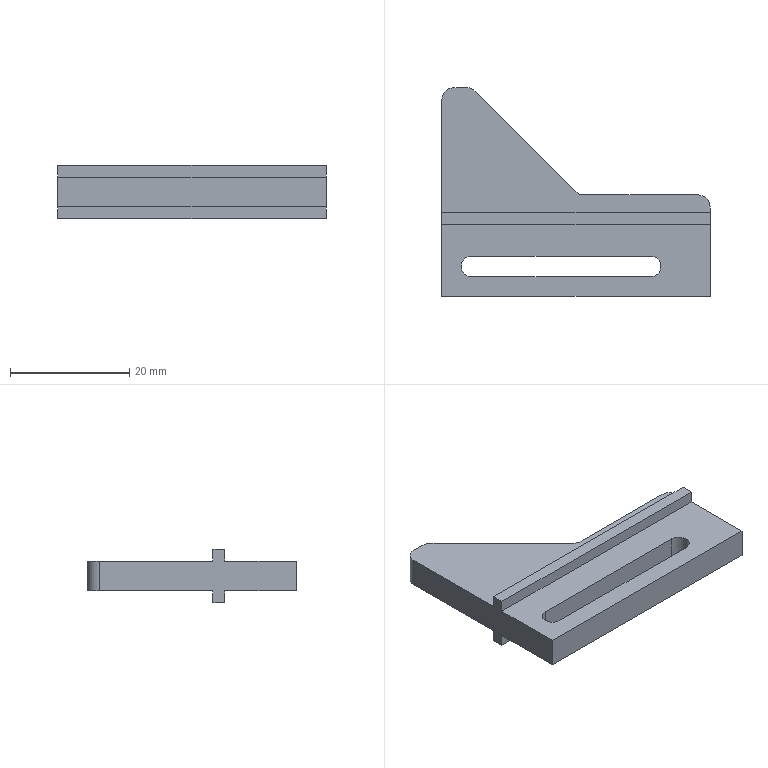Part | NX | 1 solid | 24 faces | box 45 x 35 x 9 mm | volume 4863 mm3 | plane 18 | cylinder 6 | commonest cylinder face diameters 4 x4 3.5 x2
STEP:
#1=CARTESIAN_POINT('',(-10.,-10.25,2.5));
#2=VERTEX_POINT('',#1);
#3=CARTESIAN_POINT('',(-10.,-13.75,2.5));
#4=VERTEX_POINT('',#3);
#5=CARTESIAN_POINT('',(-10.,-12.,2.5));
#6=DIRECTION('',(0.,0.,-1.));
#7=DIRECTION('',(-1.,0.,0.));
#8=AXIS2_PLACEMENT_3D('',#5,#6,#7);
#9=CIRCLE('',#8,1.75);
#10=EDGE_CURVE('',#2,#4,#9,.T.);
#11=ORIENTED_EDGE('',*,*,#10,.T.);
#12=CARTESIAN_POINT('',(-40.,-13.75,2.5));
#13=VERTEX_POINT('',#12);
#14=CARTESIAN_POINT('',(-10.,-13.75,2.5));
#15=DIRECTION('',(-1.,0.,0.));
#16=VECTOR('',#15,1000.);
#17=LINE('',#14,#16);
#18=EDGE_CURVE('',#4,#13,#17,.T.);
#19=ORIENTED_EDGE('',*,*,#18,.T.);
#20=CARTESIAN_POINT('',(-40.,-10.25,2.5));
#21=VERTEX_POINT('',#20);
#22=CARTESIAN_POINT('',(-40.,-12.,2.5));
#23=DIRECTION('',(0.,0.,-1.));
#24=DIRECTION('',(-1.,0.,0.));
#25=AXIS2_PLACEMENT_3D('',#22,#23,#24);
#26=CIRCLE('',#25,1.75);
#27=EDGE_CURVE('',#13,#21,#26,.T.);
#28=ORIENTED_EDGE('',*,*,#27,.T.);
#29=CARTESIAN_POINT('',(-10.,-10.25,2.5));
#30=DIRECTION('',(1.,0.,0.));
#31=VECTOR('',#30,1000.);
#32=LINE('',#29,#31);
#33=EDGE_CURVE('',#21,#2,#32,.T.);
#34=ORIENTED_EDGE('',*,*,#33,.T.);
#35=EDGE_LOOP('',(#11,#19,#28,#34));
#36=FACE_BOUND('',#35,.T.);
#37=CARTESIAN_POINT('',(0.,-17.,2.5));
#38=VERTEX_POINT('',#37);
#39=CARTESIAN_POINT('',(0.,-5.,2.5));
#40=VERTEX_POINT('',#39);
#41=CARTESIAN_POINT('',(0.,-17.,2.5));
#42=DIRECTION('',(0.,1.,0.));
#43=VECTOR('',#42,1000.);
#44=LINE('',#41,#43);
#45=EDGE_CURVE('',#38,#40,#44,.T.);
#46=ORIENTED_EDGE('',*,*,#45,.T.);
#47=CARTESIAN_POINT('',(-45.,-5.,2.5));
#48=VERTEX_POINT('',#47);
#49=CARTESIAN_POINT('',(0.,-5.,2.5));
#50=DIRECTION('',(-1.,0.,0.));
#51=VECTOR('',#50,1000.);
#52=LINE('',#49,#51);
#53=EDGE_CURVE('',#40,#48,#52,.T.);
#54=ORIENTED_EDGE('',*,*,#53,.T.);
#55=CARTESIAN_POINT('',(-45.,-17.,2.5));
#56=VERTEX_POINT('',#55);
#57=CARTESIAN_POINT('',(-45.,18.,2.5));
#58=DIRECTION('',(0.,-1.,0.));
#59=VECTOR('',#58,1000.);
#60=LINE('',#57,#59);
#61=EDGE_CURVE('',#48,#56,#60,.T.);
#62=ORIENTED_EDGE('',*,*,#61,.T.);
#63=CARTESIAN_POINT('',(-45.,-17.,2.5));
#64=DIRECTION('',(1.,0.,0.));
#65=VECTOR('',#64,1000.);
#66=LINE('',#63,#65);
#67=EDGE_CURVE('',#56,#38,#66,.T.);
#68=ORIENTED_EDGE('',*,*,#67,.T.);
#69=EDGE_LOOP('',(#46,#54,#62,#68));
#70=FACE_BOUND('',#69,.T.);
#71=CARTESIAN_POINT('',(0.,0.,2.5));
#72=DIRECTION('',(0.,0.,1.));
#73=DIRECTION('',(1.,0.,0.));
#74=AXIS2_PLACEMENT_3D('',#71,#72,#73);
#75=PLANE('',#74);
#76=ADVANCED_FACE('',(#36,#70),#75,.T.);
#77=CARTESIAN_POINT('',(-45.,16.,2.5));
#78=VERTEX_POINT('',#77);
#79=CARTESIAN_POINT('',(-45.,-3.,2.5));
#80=VERTEX_POINT('',#79);
#81=CARTESIAN_POINT('',(-45.,18.,2.5));
#82=DIRECTION('',(0.,-1.,0.));
#83=VECTOR('',#82,1000.);
#84=LINE('',#81,#83);
#85=EDGE_CURVE('',#78,#80,#84,.T.);
#86=ORIENTED_EDGE('',*,*,#85,.T.);
#87=CARTESIAN_POINT('',(0.,-3.,2.5));
#88=VERTEX_POINT('',#87);
#89=CARTESIAN_POINT('',(0.,-3.,2.5));
#90=DIRECTION('',(1.,0.,0.));
#91=VECTOR('',#90,1000.);
#92=LINE('',#89,#91);
#93=EDGE_CURVE('',#80,#88,#92,.T.);
#94=ORIENTED_EDGE('',*,*,#93,.T.);
#95=CARTESIAN_POINT('',(0.,-2.,2.5));
#96=VERTEX_POINT('',#95);
#97=CARTESIAN_POINT('',(0.,-17.,2.5));
#98=DIRECTION('',(0.,1.,0.));
#99=VECTOR('',#98,1000.);
#100=LINE('',#97,#99);
#101=EDGE_CURVE('',#88,#96,#100,.T.);
#102=ORIENTED_EDGE('',*,*,#101,.T.);
#103=CARTESIAN_POINT('',(-2.,0.,2.5));
#104=VERTEX_POINT('',#103);
#105=CARTESIAN_POINT('',(-2.,-2.,2.5));
#106=DIRECTION('',(0.,0.,1.));
#107=DIRECTION('',(1.,0.,0.));
#108=AXIS2_PLACEMENT_3D('',#105,#106,#107);
#109=CIRCLE('',#108,2.);
#110=EDGE_CURVE('',#96,#104,#109,.T.);
#111=ORIENTED_EDGE('',*,*,#110,.T.);
#112=CARTESIAN_POINT('',(-21.172,0.,2.5));
#113=VERTEX_POINT('',#112);
#114=CARTESIAN_POINT('',(0.,0.,2.5));
#115=DIRECTION('',(-1.,0.,0.));
#116=VECTOR('',#115,1000.);
#117=LINE('',#114,#116);
#118=EDGE_CURVE('',#104,#113,#117,.T.);
#119=ORIENTED_EDGE('',*,*,#118,.T.);
#120=CARTESIAN_POINT('',(-22.586,0.5858,2.5));
#121=VERTEX_POINT('',#120);
#122=CARTESIAN_POINT('',(-21.172,2.,2.5));
#123=DIRECTION('',(0.,0.,1.));
#124=DIRECTION('',(1.,0.,0.));
#125=AXIS2_PLACEMENT_3D('',#122,#123,#124);
#126=CIRCLE('',#125,2.);
#127=EDGE_CURVE('',#113,#121,#126,.F.);
#128=ORIENTED_EDGE('',*,*,#127,.T.);
#129=CARTESIAN_POINT('',(-39.414,17.414,2.5));
#130=VERTEX_POINT('',#129);
#131=CARTESIAN_POINT('',(-22.,0.,2.5));
#132=DIRECTION('',(-0.7071,0.7071,0.));
#133=VECTOR('',#132,1000.);
#134=LINE('',#131,#133);
#135=EDGE_CURVE('',#121,#130,#134,.T.);
#136=ORIENTED_EDGE('',*,*,#135,.T.);
#137=CARTESIAN_POINT('',(-40.828,18.,2.5));
#138=VERTEX_POINT('',#137);
#139=CARTESIAN_POINT('',(-40.828,16.,2.5));
#140=DIRECTION('',(0.,0.,1.));
#141=DIRECTION('',(1.,0.,0.));
#142=AXIS2_PLACEMENT_3D('',#139,#140,#141);
#143=CIRCLE('',#142,2.);
#144=EDGE_CURVE('',#130,#138,#143,.T.);
#145=ORIENTED_EDGE('',*,*,#144,.T.);
#146=CARTESIAN_POINT('',(-43.,18.,2.5));
#147=VERTEX_POINT('',#146);
#148=CARTESIAN_POINT('',(-40.,18.,2.5));
#149=DIRECTION('',(-1.,0.,0.));
#150=VECTOR('',#149,1000.);
#151=LINE('',#148,#150);
#152=EDGE_CURVE('',#138,#147,#151,.T.);
#153=ORIENTED_EDGE('',*,*,#152,.T.);
#154=CARTESIAN_POINT('',(-43.,16.,2.5));
#155=DIRECTION('',(0.,0.,1.));
#156=DIRECTION('',(1.,0.,0.));
#157=AXIS2_PLACEMENT_3D('',#154,#155,#156);
#158=CIRCLE('',#157,2.);
#159=EDGE_CURVE('',#147,#78,#158,.T.);
#160=ORIENTED_EDGE('',*,*,#159,.T.);
#161=EDGE_LOOP('',(#86,#94,#102,#111,#119,#128,#136,#145,#153,#160));
#162=FACE_BOUND('',#161,.T.);
#163=CARTESIAN_POINT('',(0.,0.,2.5));
#164=DIRECTION('',(0.,0.,1.));
#165=DIRECTION('',(1.,0.,0.));
#166=AXIS2_PLACEMENT_3D('',#163,#164,#165);
#167=PLANE('',#166);
#168=ADVANCED_FACE('',(#162),#167,.T.);
#169=CARTESIAN_POINT('',(-45.,-3.,-2.5));
#170=VERTEX_POINT('',#169);
#171=CARTESIAN_POINT('',(0.,-3.,-2.5));
#172=VERTEX_POINT('',#171);
#173=CARTESIAN_POINT('',(0.,-3.,-2.5));
#174=DIRECTION('',(1.,0.,0.));
#175=VECTOR('',#174,1000.);
#176=LINE('',#173,#175);
#177=EDGE_CURVE('',#170,#172,#176,.T.);
#178=ORIENTED_EDGE('',*,*,#177,.F.);
#179=CARTESIAN_POINT('',(-45.,16.,-2.5));
#180=VERTEX_POINT('',#179);
#181=CARTESIAN_POINT('',(-45.,18.,-2.5));
#182=DIRECTION('',(0.,-1.,0.));
#183=VECTOR('',#182,1000.);
#184=LINE('',#181,#183);
#185=EDGE_CURVE('',#180,#170,#184,.T.);
#186=ORIENTED_EDGE('',*,*,#185,.F.);
#187=CARTESIAN_POINT('',(-43.,18.,-2.5));
#188=VERTEX_POINT('',#187);
#189=CARTESIAN_POINT('',(-43.,16.,-2.5));
#190=DIRECTION('',(0.,0.,1.));
#191=DIRECTION('',(1.,0.,0.));
#192=AXIS2_PLACEMENT_3D('',#189,#190,#191);
#193=CIRCLE('',#192,2.);
#194=EDGE_CURVE('',#180,#188,#193,.F.);
#195=ORIENTED_EDGE('',*,*,#194,.T.);
#196=CARTESIAN_POINT('',(-40.828,18.,-2.5));
#197=VERTEX_POINT('',#196);
#198=CARTESIAN_POINT('',(-40.,18.,-2.5));
#199=DIRECTION('',(-1.,0.,0.));
#200=VECTOR('',#199,1000.);
#201=LINE('',#198,#200);
#202=EDGE_CURVE('',#197,#188,#201,.T.);
#203=ORIENTED_EDGE('',*,*,#202,.F.);
#204=CARTESIAN_POINT('',(-39.414,17.414,-2.5));
#205=VERTEX_POINT('',#204);
#206=CARTESIAN_POINT('',(-40.828,16.,-2.5));
#207=DIRECTION('',(0.,0.,1.));
#208=DIRECTION('',(1.,0.,0.));
#209=AXIS2_PLACEMENT_3D('',#206,#207,#208);
#210=CIRCLE('',#209,2.);
#211=EDGE_CURVE('',#197,#205,#210,.F.);
#212=ORIENTED_EDGE('',*,*,#211,.T.);
#213=CARTESIAN_POINT('',(-22.586,0.5858,-2.5));
#214=VERTEX_POINT('',#213);
#215=CARTESIAN_POINT('',(-22.,0.,-2.5));
#216=DIRECTION('',(-0.7071,0.7071,0.));
#217=VECTOR('',#216,1000.);
#218=LINE('',#215,#217);
#219=EDGE_CURVE('',#214,#205,#218,.T.);
#220=ORIENTED_EDGE('',*,*,#219,.F.);
#221=CARTESIAN_POINT('',(-21.172,0.,-2.5));
#222=VERTEX_POINT('',#221);
#223=CARTESIAN_POINT('',(-21.172,2.,-2.5));
#224=DIRECTION('',(0.,0.,1.));
#225=DIRECTION('',(1.,0.,0.));
#226=AXIS2_PLACEMENT_3D('',#223,#224,#225);
#227=CIRCLE('',#226,2.);
#228=EDGE_CURVE('',#214,#222,#227,.T.);
#229=ORIENTED_EDGE('',*,*,#228,.T.);
#230=CARTESIAN_POINT('',(-2.,0.,-2.5));
#231=VERTEX_POINT('',#230);
#232=CARTESIAN_POINT('',(0.,0.,-2.5));
#233=DIRECTION('',(-1.,0.,0.));
#234=VECTOR('',#233,1000.);
#235=LINE('',#232,#234);
#236=EDGE_CURVE('',#231,#222,#235,.T.);
#237=ORIENTED_EDGE('',*,*,#236,.F.);
#238=CARTESIAN_POINT('',(0.,-2.,-2.5));
#239=VERTEX_POINT('',#238);
#240=CARTESIAN_POINT('',(-2.,-2.,-2.5));
#241=DIRECTION('',(0.,0.,1.));
#242=DIRECTION('',(1.,0.,0.));
#243=AXIS2_PLACEMENT_3D('',#240,#241,#242);
#244=CIRCLE('',#243,2.);
#245=EDGE_CURVE('',#231,#239,#244,.F.);
#246=ORIENTED_EDGE('',*,*,#245,.T.);
#247=CARTESIAN_POINT('',(0.,-17.,-2.5));
#248=DIRECTION('',(0.,1.,0.));
#249=VECTOR('',#248,1000.);
#250=LINE('',#247,#249);
#251=EDGE_CURVE('',#172,#239,#250,.T.);
#252=ORIENTED_EDGE('',*,*,#251,.F.);
#253=EDGE_LOOP('',(#178,#186,#195,#203,#212,#220,#229,#237,#246,#252));
#254=FACE_BOUND('',#253,.T.);
#255=CARTESIAN_POINT('',(0.,0.,-2.5));
#256=DIRECTION('',(0.,0.,1.));
#257=DIRECTION('',(1.,0.,0.));
#258=AXIS2_PLACEMENT_3D('',#255,#256,#257);
#259=PLANE('',#258);
#260=ADVANCED_FACE('',(#254),#259,.F.);
#261=CARTESIAN_POINT('',(-10.,-13.75,-2.5));
#262=VERTEX_POINT('',#261);
#263=CARTESIAN_POINT('',(-40.,-13.75,-2.5));
#264=VERTEX_POINT('',#263);
#265=CARTESIAN_POINT('',(-10.,-13.75,-2.5));
#266=DIRECTION('',(-1.,0.,0.));
#267=VECTOR('',#266,1000.);
#268=LINE('',#265,#267);
#269=EDGE_CURVE('',#262,#264,#268,.T.);
#270=ORIENTED_EDGE('',*,*,#269,.F.);
#271=CARTESIAN_POINT('',(-10.,-10.25,-2.5));
#272=VERTEX_POINT('',#271);
#273=CARTESIAN_POINT('',(-10.,-12.,-2.5));
#274=DIRECTION('',(0.,0.,-1.));
#275=DIRECTION('',(-1.,0.,0.));
#276=AXIS2_PLACEMENT_3D('',#273,#274,#275);
#277=CIRCLE('',#276,1.75);
#278=EDGE_CURVE('',#272,#262,#277,.T.);
#279=ORIENTED_EDGE('',*,*,#278,.F.);
#280=CARTESIAN_POINT('',(-40.,-10.25,-2.5));
#281=VERTEX_POINT('',#280);
#282=CARTESIAN_POINT('',(-10.,-10.25,-2.5));
#283=DIRECTION('',(1.,0.,0.));
#284=VECTOR('',#283,1000.);
#285=LINE('',#282,#284);
#286=EDGE_CURVE('',#281,#272,#285,.T.);
#287=ORIENTED_EDGE('',*,*,#286,.F.);
#288=CARTESIAN_POINT('',(-40.,-12.,-2.5));
#289=DIRECTION('',(0.,0.,-1.));
#290=DIRECTION('',(-1.,0.,0.));
#291=AXIS2_PLACEMENT_3D('',#288,#289,#290);
#292=CIRCLE('',#291,1.75);
#293=EDGE_CURVE('',#264,#281,#292,.T.);
#294=ORIENTED_EDGE('',*,*,#293,.F.);
#295=EDGE_LOOP('',(#270,#279,#287,#294));
#296=FACE_BOUND('',#295,.T.);
#297=CARTESIAN_POINT('',(0.,-5.,-2.5));
#298=VERTEX_POINT('',#297);
#299=CARTESIAN_POINT('',(-45.,-5.,-2.5));
#300=VERTEX_POINT('',#299);
#301=CARTESIAN_POINT('',(0.,-5.,-2.5));
#302=DIRECTION('',(-1.,0.,0.));
#303=VECTOR('',#302,1000.);
#304=LINE('',#301,#303);
#305=EDGE_CURVE('',#298,#300,#304,.T.);
#306=ORIENTED_EDGE('',*,*,#305,.F.);
#307=CARTESIAN_POINT('',(0.,-17.,-2.5));
#308=VERTEX_POINT('',#307);
#309=CARTESIAN_POINT('',(0.,-17.,-2.5));
#310=DIRECTION('',(0.,1.,0.));
#311=VECTOR('',#310,1000.);
#312=LINE('',#309,#311);
#313=EDGE_CURVE('',#308,#298,#312,.T.);
#314=ORIENTED_EDGE('',*,*,#313,.F.);
#315=CARTESIAN_POINT('',(-45.,-17.,-2.5));
#316=VERTEX_POINT('',#315);
#317=CARTESIAN_POINT('',(-45.,-17.,-2.5));
#318=DIRECTION('',(1.,0.,0.));
#319=VECTOR('',#318,1000.);
#320=LINE('',#317,#319);
#321=EDGE_CURVE('',#316,#308,#320,.T.);
#322=ORIENTED_EDGE('',*,*,#321,.F.);
#323=CARTESIAN_POINT('',(-45.,18.,-2.5));
#324=DIRECTION('',(0.,-1.,0.));
#325=VECTOR('',#324,1000.);
#326=LINE('',#323,#325);
#327=EDGE_CURVE('',#300,#316,#326,.T.);
#328=ORIENTED_EDGE('',*,*,#327,.F.);
#329=EDGE_LOOP('',(#306,#314,#322,#328));
#330=FACE_BOUND('',#329,.T.);
#331=CARTESIAN_POINT('',(0.,0.,-2.5));
#332=DIRECTION('',(0.,0.,1.));
#333=DIRECTION('',(1.,0.,0.));
#334=AXIS2_PLACEMENT_3D('',#331,#332,#333);
#335=PLANE('',#334);
#336=ADVANCED_FACE('',(#296,#330),#335,.F.);
#337=ORIENTED_EDGE('',*,*,#313,.T.);
#338=CARTESIAN_POINT('',(0.,-5.,-4.5));
#339=VERTEX_POINT('',#338);
#340=CARTESIAN_POINT('',(0.,-5.,-4.5));
#341=DIRECTION('',(0.,0.,1.));
#342=VECTOR('',#341,1000.);
#343=LINE('',#340,#342);
#344=EDGE_CURVE('',#339,#298,#343,.T.);
#345=ORIENTED_EDGE('',*,*,#344,.F.);
#346=CARTESIAN_POINT('',(0.,-3.,-4.5));
#347=VERTEX_POINT('',#346);
#348=CARTESIAN_POINT('',(0.,-3.,-4.5));
#349=DIRECTION('',(0.,-1.,0.));
#350=VECTOR('',#349,1000.);
#351=LINE('',#348,#350);
#352=EDGE_CURVE('',#347,#339,#351,.T.);
#353=ORIENTED_EDGE('',*,*,#352,.F.);
#354=CARTESIAN_POINT('',(0.,-3.,-4.5));
#355=DIRECTION('',(0.,0.,1.));
#356=VECTOR('',#355,1000.);
#357=LINE('',#354,#356);
#358=EDGE_CURVE('',#347,#172,#357,.T.);
#359=ORIENTED_EDGE('',*,*,#358,.T.);
#360=ORIENTED_EDGE('',*,*,#251,.T.);
#361=CARTESIAN_POINT('',(0.,-2.,2.5));
#362=DIRECTION('',(0.,0.,-1.));
#363=VECTOR('',#362,1000.);
#364=LINE('',#361,#363);
#365=EDGE_CURVE('',#239,#96,#364,.F.);
#366=ORIENTED_EDGE('',*,*,#365,.T.);
#367=ORIENTED_EDGE('',*,*,#101,.F.);
#368=CARTESIAN_POINT('',(0.,-3.,4.5));
#369=VERTEX_POINT('',#368);
#370=CARTESIAN_POINT('',(0.,-3.,4.5));
#371=DIRECTION('',(0.,0.,-1.));
#372=VECTOR('',#371,1000.);
#373=LINE('',#370,#372);
#374=EDGE_CURVE('',#369,#88,#373,.T.);
#375=ORIENTED_EDGE('',*,*,#374,.F.);
#376=CARTESIAN_POINT('',(0.,-5.,4.5));
#377=VERTEX_POINT('',#376);
#378=CARTESIAN_POINT('',(0.,-3.,4.5));
#379=DIRECTION('',(0.,-1.,0.));
#380=VECTOR('',#379,1000.);
#381=LINE('',#378,#380);
#382=EDGE_CURVE('',#369,#377,#381,.T.);
#383=ORIENTED_EDGE('',*,*,#382,.T.);
#384=CARTESIAN_POINT('',(0.,-5.,4.5));
#385=DIRECTION('',(0.,0.,-1.));
#386=VECTOR('',#385,1000.);
#387=LINE('',#384,#386);
#388=EDGE_CURVE('',#377,#40,#387,.T.);
#389=ORIENTED_EDGE('',*,*,#388,.T.);
#390=ORIENTED_EDGE('',*,*,#45,.F.);
#391=CARTESIAN_POINT('',(0.,-17.,2.5));
#392=DIRECTION('',(0.,0.,-1.));
#393=VECTOR('',#392,1000.);
#394=LINE('',#391,#393);
#395=EDGE_CURVE('',#38,#308,#394,.T.);
#396=ORIENTED_EDGE('',*,*,#395,.T.);
#397=EDGE_LOOP('',(#337,#345,#353,#359,#360,#366,#367,#375,#383,#389,#390,#396));
#398=FACE_BOUND('',#397,.T.);
#399=CARTESIAN_POINT('',(0.,-17.,2.5));
#400=DIRECTION('',(-1.,0.,0.));
#401=DIRECTION('',(0.,0.,1.));
#402=AXIS2_PLACEMENT_3D('',#399,#400,#401);
#403=PLANE('',#402);
#404=ADVANCED_FACE('',(#398),#403,.F.);
#405=ORIENTED_EDGE('',*,*,#118,.F.);
#406=CARTESIAN_POINT('',(-2.,0.,2.5));
#407=DIRECTION('',(0.,0.,-1.));
#408=VECTOR('',#407,1000.);
#409=LINE('',#406,#408);
#410=EDGE_CURVE('',#104,#231,#409,.T.);
#411=ORIENTED_EDGE('',*,*,#410,.T.);
#412=ORIENTED_EDGE('',*,*,#236,.T.);
#413=CARTESIAN_POINT('',(-21.172,0.,2.5));
#414=DIRECTION('',(0.,0.,-1.));
#415=VECTOR('',#414,1000.);
#416=LINE('',#413,#415);
#417=EDGE_CURVE('',#222,#113,#416,.F.);
#418=ORIENTED_EDGE('',*,*,#417,.T.);
#419=EDGE_LOOP('',(#405,#411,#412,#418));
#420=FACE_BOUND('',#419,.T.);
#421=CARTESIAN_POINT('',(0.,0.,2.5));
#422=DIRECTION('',(0.,-1.,0.));
#423=DIRECTION('',(1.,0.,0.));
#424=AXIS2_PLACEMENT_3D('',#421,#422,#423);
#425=PLANE('',#424);
#426=ADVANCED_FACE('',(#420),#425,.F.);
#427=ORIENTED_EDGE('',*,*,#219,.T.);
#428=CARTESIAN_POINT('',(-39.414,17.414,2.5));
#429=DIRECTION('',(0.,0.,-1.));
#430=VECTOR('',#429,1000.);
#431=LINE('',#428,#430);
#432=EDGE_CURVE('',#205,#130,#431,.F.);
#433=ORIENTED_EDGE('',*,*,#432,.T.);
#434=ORIENTED_EDGE('',*,*,#135,.F.);
#435=CARTESIAN_POINT('',(-22.586,0.5858,-2.5));
#436=DIRECTION('',(0.,0.,-1.));
#437=VECTOR('',#436,1000.);
#438=LINE('',#435,#437);
#439=EDGE_CURVE('',#121,#214,#438,.T.);
#440=ORIENTED_EDGE('',*,*,#439,.T.);
#441=EDGE_LOOP('',(#427,#433,#434,#440));
#442=FACE_BOUND('',#441,.T.);
#443=CARTESIAN_POINT('',(-22.,0.,2.5));
#444=DIRECTION('',(-0.7071,-0.7071,0.));
#445=DIRECTION('',(0.7071,-0.7071,0.));
#446=AXIS2_PLACEMENT_3D('',#443,#444,#445);
#447=PLANE('',#446);
#448=ADVANCED_FACE('',(#442),#447,.F.);
#449=ORIENTED_EDGE('',*,*,#202,.T.);
#450=CARTESIAN_POINT('',(-43.,18.,2.5));
#451=DIRECTION('',(0.,0.,-1.));
#452=VECTOR('',#451,1000.);
#453=LINE('',#450,#452);
#454=EDGE_CURVE('',#188,#147,#453,.F.);
#455=ORIENTED_EDGE('',*,*,#454,.T.);
#456=ORIENTED_EDGE('',*,*,#152,.F.);
#457=CARTESIAN_POINT('',(-40.828,18.,2.5));
#458=DIRECTION('',(0.,0.,-1.));
#459=VECTOR('',#458,1000.);
#460=LINE('',#457,#459);
#461=EDGE_CURVE('',#138,#197,#460,.T.);
#462=ORIENTED_EDGE('',*,*,#461,.T.);
#463=EDGE_LOOP('',(#449,#455,#456,#462));
#464=FACE_BOUND('',#463,.T.);
#465=CARTESIAN_POINT('',(-40.,18.,2.5));
#466=DIRECTION('',(0.,-1.,0.));
#467=DIRECTION('',(1.,0.,0.));
#468=AXIS2_PLACEMENT_3D('',#465,#466,#467);
#469=PLANE('',#468);
#470=ADVANCED_FACE('',(#464),#469,.F.);
#471=ORIENTED_EDGE('',*,*,#85,.F.);
#472=CARTESIAN_POINT('',(-45.,16.,2.5));
#473=DIRECTION('',(0.,0.,-1.));
#474=VECTOR('',#473,1000.);
#475=LINE('',#472,#474);
#476=EDGE_CURVE('',#78,#180,#475,.T.);
#477=ORIENTED_EDGE('',*,*,#476,.T.);
#478=ORIENTED_EDGE('',*,*,#185,.T.);
#479=CARTESIAN_POINT('',(-45.,-3.,-4.5));
#480=VERTEX_POINT('',#479);
#481=CARTESIAN_POINT('',(-45.,-3.,-4.5));
#482=DIRECTION('',(0.,0.,1.));
#483=VECTOR('',#482,1000.);
#484=LINE('',#481,#483);
#485=EDGE_CURVE('',#480,#170,#484,.T.);
#486=ORIENTED_EDGE('',*,*,#485,.F.);
#487=CARTESIAN_POINT('',(-45.,-5.,-4.5));
#488=VERTEX_POINT('',#487);
#489=CARTESIAN_POINT('',(-45.,-3.,-4.5));
#490=DIRECTION('',(0.,1.,0.));
#491=VECTOR('',#490,1000.);
#492=LINE('',#489,#491);
#493=EDGE_CURVE('',#488,#480,#492,.T.);
#494=ORIENTED_EDGE('',*,*,#493,.F.);
#495=CARTESIAN_POINT('',(-45.,-5.,-4.5));
#496=DIRECTION('',(0.,0.,1.));
#497=VECTOR('',#496,1000.);
#498=LINE('',#495,#497);
#499=EDGE_CURVE('',#488,#300,#498,.T.);
#500=ORIENTED_EDGE('',*,*,#499,.T.);
#501=ORIENTED_EDGE('',*,*,#327,.T.);
#502=CARTESIAN_POINT('',(-45.,-17.,2.5));
#503=DIRECTION('',(0.,0.,-1.));
#504=VECTOR('',#503,1000.);
#505=LINE('',#502,#504);
#506=EDGE_CURVE('',#56,#316,#505,.T.);
#507=ORIENTED_EDGE('',*,*,#506,.F.);
#508=ORIENTED_EDGE('',*,*,#61,.F.);
#509=CARTESIAN_POINT('',(-45.,-5.,4.5));
#510=VERTEX_POINT('',#509);
#511=CARTESIAN_POINT('',(-45.,-5.,4.5));
#512=DIRECTION('',(0.,0.,-1.));
#513=VECTOR('',#512,1000.);
#514=LINE('',#511,#513);
#515=EDGE_CURVE('',#510,#48,#514,.T.);
#516=ORIENTED_EDGE('',*,*,#515,.F.);
#517=CARTESIAN_POINT('',(-45.,-3.,4.5));
#518=VERTEX_POINT('',#517);
#519=CARTESIAN_POINT('',(-45.,-3.,4.5));
#520=DIRECTION('',(0.,1.,0.));
#521=VECTOR('',#520,1000.);
#522=LINE('',#519,#521);
#523=EDGE_CURVE('',#510,#518,#522,.T.);
#524=ORIENTED_EDGE('',*,*,#523,.T.);
#525=CARTESIAN_POINT('',(-45.,-3.,4.5));
#526=DIRECTION('',(0.,0.,-1.));
#527=VECTOR('',#526,1000.);
#528=LINE('',#525,#527);
#529=EDGE_CURVE('',#518,#80,#528,.T.);
#530=ORIENTED_EDGE('',*,*,#529,.T.);
#531=EDGE_LOOP('',(#471,#477,#478,#486,#494,#500,#501,#507,#508,#516,#524,#530));
#532=FACE_BOUND('',#531,.T.);
#533=CARTESIAN_POINT('',(-45.,18.,2.5));
#534=DIRECTION('',(1.,0.,0.));
#535=DIRECTION('',(0.,0.,-1.));
#536=AXIS2_PLACEMENT_3D('',#533,#534,#535);
#537=PLANE('',#536);
#538=ADVANCED_FACE('',(#532),#537,.F.);
#539=ORIENTED_EDGE('',*,*,#321,.T.);
#540=ORIENTED_EDGE('',*,*,#395,.F.);
#541=ORIENTED_EDGE('',*,*,#67,.F.);
#542=ORIENTED_EDGE('',*,*,#506,.T.);
#543=EDGE_LOOP('',(#539,#540,#541,#542));
#544=FACE_BOUND('',#543,.T.);
#545=CARTESIAN_POINT('',(-45.,-17.,2.5));
#546=DIRECTION('',(0.,1.,0.));
#547=DIRECTION('',(0.,0.,1.));
#548=AXIS2_PLACEMENT_3D('',#545,#546,#547);
#549=PLANE('',#548);
#550=ADVANCED_FACE('',(#544),#549,.F.);
#551=ORIENTED_EDGE('',*,*,#278,.T.);
#552=CARTESIAN_POINT('',(-10.,-13.75,2.5));
#553=DIRECTION('',(0.,0.,-1.));
#554=VECTOR('',#553,1000.);
#555=LINE('',#552,#554);
#556=EDGE_CURVE('',#4,#262,#555,.T.);
#557=ORIENTED_EDGE('',*,*,#556,.F.);
#558=ORIENTED_EDGE('',*,*,#10,.F.);
#559=CARTESIAN_POINT('',(-10.,-10.25,2.5));
#560=DIRECTION('',(0.,0.,-1.));
#561=VECTOR('',#560,1000.);
#562=LINE('',#559,#561);
#563=EDGE_CURVE('',#2,#272,#562,.T.);
#564=ORIENTED_EDGE('',*,*,#563,.T.);
#565=EDGE_LOOP('',(#551,#557,#558,#564));
#566=FACE_BOUND('',#565,.T.);
#567=CARTESIAN_POINT('',(-10.,-12.,2.5));
#568=DIRECTION('',(0.,0.,-1.));
#569=DIRECTION('',(-1.,0.,0.));
#570=AXIS2_PLACEMENT_3D('',#567,#568,#569);
#571=CYLINDRICAL_SURFACE('',#570,1.75);
#572=ADVANCED_FACE('',(#566),#571,.F.);
#573=ORIENTED_EDGE('',*,*,#286,.T.);
#574=ORIENTED_EDGE('',*,*,#563,.F.);
#575=ORIENTED_EDGE('',*,*,#33,.F.);
#576=CARTESIAN_POINT('',(-40.,-10.25,2.5));
#577=DIRECTION('',(0.,0.,-1.));
#578=VECTOR('',#577,1000.);
#579=LINE('',#576,#578);
#580=EDGE_CURVE('',#21,#281,#579,.T.);
#581=ORIENTED_EDGE('',*,*,#580,.T.);
#582=EDGE_LOOP('',(#573,#574,#575,#581));
#583=FACE_BOUND('',#582,.T.);
#584=CARTESIAN_POINT('',(-10.,-10.25,2.5));
#585=DIRECTION('',(0.,1.,0.));
#586=DIRECTION('',(0.,0.,1.));
#587=AXIS2_PLACEMENT_3D('',#584,#585,#586);
#588=PLANE('',#587);
#589=ADVANCED_FACE('',(#583),#588,.F.);
#590=ORIENTED_EDGE('',*,*,#293,.T.);
#591=ORIENTED_EDGE('',*,*,#580,.F.);
#592=ORIENTED_EDGE('',*,*,#27,.F.);
#593=CARTESIAN_POINT('',(-40.,-13.75,2.5));
#594=DIRECTION('',(0.,0.,-1.));
#595=VECTOR('',#594,1000.);
#596=LINE('',#593,#595);
#597=EDGE_CURVE('',#13,#264,#596,.T.);
#598=ORIENTED_EDGE('',*,*,#597,.T.);
#599=EDGE_LOOP('',(#590,#591,#592,#598));
#600=FACE_BOUND('',#599,.T.);
#601=CARTESIAN_POINT('',(-40.,-12.,2.5));
#602=DIRECTION('',(0.,0.,-1.));
#603=DIRECTION('',(-1.,0.,0.));
#604=AXIS2_PLACEMENT_3D('',#601,#602,#603);
#605=CYLINDRICAL_SURFACE('',#604,1.75);
#606=ADVANCED_FACE('',(#600),#605,.F.);
#607=ORIENTED_EDGE('',*,*,#269,.T.);
#608=ORIENTED_EDGE('',*,*,#597,.F.);
#609=ORIENTED_EDGE('',*,*,#18,.F.);
#610=ORIENTED_EDGE('',*,*,#556,.T.);
#611=EDGE_LOOP('',(#607,#608,#609,#610));
#612=FACE_BOUND('',#611,.T.);
#613=CARTESIAN_POINT('',(-10.,-13.75,2.5));
#614=DIRECTION('',(0.,-1.,0.));
#615=DIRECTION('',(0.,0.,-1.));
#616=AXIS2_PLACEMENT_3D('',#613,#614,#615);
#617=PLANE('',#616);
#618=ADVANCED_FACE('',(#612),#617,.F.);
#619=ORIENTED_EDGE('',*,*,#110,.F.);
#620=ORIENTED_EDGE('',*,*,#365,.F.);
#621=ORIENTED_EDGE('',*,*,#245,.F.);
#622=ORIENTED_EDGE('',*,*,#410,.F.);
#623=EDGE_LOOP('',(#619,#620,#621,#622));
#624=FACE_BOUND('',#623,.T.);
#625=CARTESIAN_POINT('',(-2.,-2.,2.5));
#626=DIRECTION('',(0.,0.,-1.));
#627=DIRECTION('',(-1.,0.,0.));
#628=AXIS2_PLACEMENT_3D('',#625,#626,#627);
#629=CYLINDRICAL_SURFACE('',#628,2.);
#630=ADVANCED_FACE('',(#624),#629,.T.);
#631=ORIENTED_EDGE('',*,*,#159,.F.);
#632=ORIENTED_EDGE('',*,*,#454,.F.);
#633=ORIENTED_EDGE('',*,*,#194,.F.);
#634=ORIENTED_EDGE('',*,*,#476,.F.);
#635=EDGE_LOOP('',(#631,#632,#633,#634));
#636=FACE_BOUND('',#635,.T.);
#637=CARTESIAN_POINT('',(-43.,16.,2.5));
#638=DIRECTION('',(0.,0.,-1.));
#639=DIRECTION('',(-1.,0.,0.));
#640=AXIS2_PLACEMENT_3D('',#637,#638,#639);
#641=CYLINDRICAL_SURFACE('',#640,2.);
#642=ADVANCED_FACE('',(#636),#641,.T.);
#643=ORIENTED_EDGE('',*,*,#144,.F.);
#644=ORIENTED_EDGE('',*,*,#432,.F.);
#645=ORIENTED_EDGE('',*,*,#211,.F.);
#646=ORIENTED_EDGE('',*,*,#461,.F.);
#647=EDGE_LOOP('',(#643,#644,#645,#646));
#648=FACE_BOUND('',#647,.T.);
#649=CARTESIAN_POINT('',(-40.828,16.,2.5));
#650=DIRECTION('',(0.,0.,-1.));
#651=DIRECTION('',(-1.,0.,0.));
#652=AXIS2_PLACEMENT_3D('',#649,#650,#651);
#653=CYLINDRICAL_SURFACE('',#652,2.);
#654=ADVANCED_FACE('',(#648),#653,.T.);
#655=ORIENTED_EDGE('',*,*,#127,.F.);
#656=ORIENTED_EDGE('',*,*,#417,.F.);
#657=ORIENTED_EDGE('',*,*,#228,.F.);
#658=ORIENTED_EDGE('',*,*,#439,.F.);
#659=EDGE_LOOP('',(#655,#656,#657,#658));
#660=FACE_BOUND('',#659,.T.);
#661=CARTESIAN_POINT('',(-21.172,2.,2.5));
#662=DIRECTION('',(0.,0.,1.));
#663=DIRECTION('',(1.,0.,0.));
#664=AXIS2_PLACEMENT_3D('',#661,#662,#663);
#665=CYLINDRICAL_SURFACE('',#664,2.);
#666=ADVANCED_FACE('',(#660),#665,.F.);
#667=ORIENTED_EDGE('',*,*,#305,.T.);
#668=ORIENTED_EDGE('',*,*,#499,.F.);
#669=CARTESIAN_POINT('',(0.,-5.,-4.5));
#670=DIRECTION('',(-1.,0.,0.));
#671=VECTOR('',#670,1000.);
#672=LINE('',#669,#671);
#673=EDGE_CURVE('',#339,#488,#672,.T.);
#674=ORIENTED_EDGE('',*,*,#673,.F.);
#675=ORIENTED_EDGE('',*,*,#344,.T.);
#676=EDGE_LOOP('',(#667,#668,#674,#675));
#677=FACE_BOUND('',#676,.T.);
#678=CARTESIAN_POINT('',(0.,-5.,-4.5));
#679=DIRECTION('',(0.,1.,0.));
#680=DIRECTION('',(0.,0.,1.));
#681=AXIS2_PLACEMENT_3D('',#678,#679,#680);
#682=PLANE('',#681);
#683=ADVANCED_FACE('',(#677),#682,.F.);
#684=ORIENTED_EDGE('',*,*,#177,.T.);
#685=ORIENTED_EDGE('',*,*,#358,.F.);
#686=CARTESIAN_POINT('',(0.,-3.,-4.5));
#687=DIRECTION('',(1.,0.,0.));
#688=VECTOR('',#687,1000.);
#689=LINE('',#686,#688);
#690=EDGE_CURVE('',#480,#347,#689,.T.);
#691=ORIENTED_EDGE('',*,*,#690,.F.);
#692=ORIENTED_EDGE('',*,*,#485,.T.);
#693=EDGE_LOOP('',(#684,#685,#691,#692));
#694=FACE_BOUND('',#693,.T.);
#695=CARTESIAN_POINT('',(0.,-3.,-4.5));
#696=DIRECTION('',(0.,-1.,0.));
#697=DIRECTION('',(0.,0.,-1.));
#698=AXIS2_PLACEMENT_3D('',#695,#696,#697);
#699=PLANE('',#698);
#700=ADVANCED_FACE('',(#694),#699,.F.);
#701=ORIENTED_EDGE('',*,*,#352,.T.);
#702=ORIENTED_EDGE('',*,*,#673,.T.);
#703=ORIENTED_EDGE('',*,*,#493,.T.);
#704=ORIENTED_EDGE('',*,*,#690,.T.);
#705=EDGE_LOOP('',(#701,#702,#703,#704));
#706=FACE_BOUND('',#705,.T.);
#707=CARTESIAN_POINT('',(0.,0.,-4.5));
#708=DIRECTION('',(0.,0.,-1.));
#709=DIRECTION('',(-1.,0.,0.));
#710=AXIS2_PLACEMENT_3D('',#707,#708,#709);
#711=PLANE('',#710);
#712=ADVANCED_FACE('',(#706),#711,.T.);
#713=ORIENTED_EDGE('',*,*,#93,.F.);
#714=ORIENTED_EDGE('',*,*,#529,.F.);
#715=CARTESIAN_POINT('',(0.,-3.,4.5));
#716=DIRECTION('',(1.,0.,0.));
#717=VECTOR('',#716,1000.);
#718=LINE('',#715,#717);
#719=EDGE_CURVE('',#518,#369,#718,.T.);
#720=ORIENTED_EDGE('',*,*,#719,.T.);
#721=ORIENTED_EDGE('',*,*,#374,.T.);
#722=EDGE_LOOP('',(#713,#714,#720,#721));
#723=FACE_BOUND('',#722,.T.);
#724=CARTESIAN_POINT('',(0.,-3.,4.5));
#725=DIRECTION('',(0.,1.,0.));
#726=DIRECTION('',(0.,0.,1.));
#727=AXIS2_PLACEMENT_3D('',#724,#725,#726);
#728=PLANE('',#727);
#729=ADVANCED_FACE('',(#723),#728,.T.);
#730=ORIENTED_EDGE('',*,*,#53,.F.);
#731=ORIENTED_EDGE('',*,*,#388,.F.);
#732=CARTESIAN_POINT('',(0.,-5.,4.5));
#733=DIRECTION('',(-1.,0.,0.));
#734=VECTOR('',#733,1000.);
#735=LINE('',#732,#734);
#736=EDGE_CURVE('',#377,#510,#735,.T.);
#737=ORIENTED_EDGE('',*,*,#736,.T.);
#738=ORIENTED_EDGE('',*,*,#515,.T.);
#739=EDGE_LOOP('',(#730,#731,#737,#738));
#740=FACE_BOUND('',#739,.T.);
#741=CARTESIAN_POINT('',(0.,-5.,4.5));
#742=DIRECTION('',(0.,-1.,0.));
#743=DIRECTION('',(0.,0.,-1.));
#744=AXIS2_PLACEMENT_3D('',#741,#742,#743);
#745=PLANE('',#744);
#746=ADVANCED_FACE('',(#740),#745,.T.);
#747=ORIENTED_EDGE('',*,*,#382,.F.);
#748=ORIENTED_EDGE('',*,*,#719,.F.);
#749=ORIENTED_EDGE('',*,*,#523,.F.);
#750=ORIENTED_EDGE('',*,*,#736,.F.);
#751=EDGE_LOOP('',(#747,#748,#749,#750));
#752=FACE_BOUND('',#751,.T.);
#753=CARTESIAN_POINT('',(0.,0.,4.5));
#754=DIRECTION('',(0.,0.,1.));
#755=DIRECTION('',(-1.,0.,0.));
#756=AXIS2_PLACEMENT_3D('',#753,#754,#755);
#757=PLANE('',#756);
#758=ADVANCED_FACE('',(#752),#757,.T.);
#759=CLOSED_SHELL('',(#76,#168,#260,#336,#404,#426,#448,#470,#538,#550,#572,#589,#606,#618,#630,#642,#654,#666,#683,#700,#712,#729,#746,#758));
#760=MANIFOLD_SOLID_BREP('',#759);
#761=(LENGTH_UNIT()NAMED_UNIT(*)SI_UNIT(.MILLI.,.METRE.));
#762=UNCERTAINTY_MEASURE_WITH_UNIT(LENGTH_MEASURE(0.00001),#761,'','');
#763=(NAMED_UNIT(*)PLANE_ANGLE_UNIT()SI_UNIT($,.RADIAN.));
#764=(NAMED_UNIT(*)SI_UNIT($,.STERADIAN.)SOLID_ANGLE_UNIT());
#765=(GEOMETRIC_REPRESENTATION_CONTEXT(3)GLOBAL_UNCERTAINTY_ASSIGNED_CONTEXT((#762))GLOBAL_UNIT_ASSIGNED_CONTEXT((#761,#763,#764))REPRESENTATION_CONTEXT('',''));
#766=ADVANCED_BREP_SHAPE_REPRESENTATION('',(#760),#765);